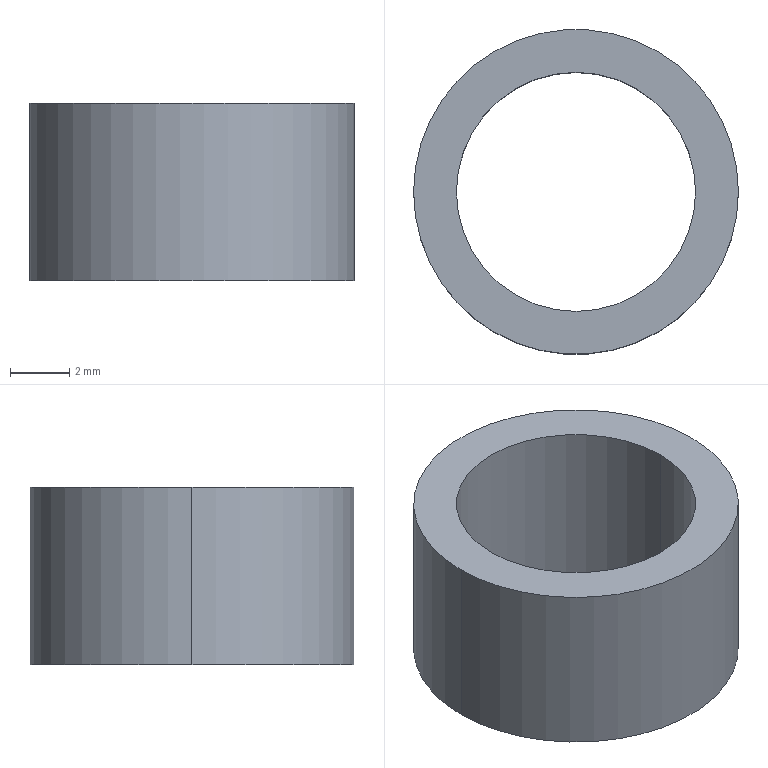Part | NX | features BREP 1 | 1 solid | 6 faces | box 11 x 11 x 6 mm | volume 261.019 mm3 | cylinder 4 | plane 2 | commonest cylinder face diameters 8.1 x2 11 x2
STEP:
#1=CARTESIAN_POINT('',(4.05,0.,6.));
#2=VERTEX_POINT('',#1);
#3=CARTESIAN_POINT('',(4.05,0.,0.));
#4=VERTEX_POINT('',#3);
#5=CARTESIAN_POINT('',(4.05,0.,6.));
#6=DIRECTION('',(0.,0.,-1.));
#7=VECTOR('',#6,1000.);
#8=LINE('',#5,#7);
#9=EDGE_CURVE('',#2,#4,#8,.T.);
#10=ORIENTED_EDGE('',*,*,#9,.F.);
#11=CARTESIAN_POINT('',(-4.05,0.,6.));
#12=VERTEX_POINT('',#11);
#13=CARTESIAN_POINT('',(0.,0.,6.));
#14=DIRECTION('',(0.,0.,1.));
#15=DIRECTION('',(1.,0.,0.));
#16=AXIS2_PLACEMENT_3D('',#13,#14,#15);
#17=CIRCLE('',#16,4.05);
#18=EDGE_CURVE('',#2,#12,#17,.T.);
#19=ORIENTED_EDGE('',*,*,#18,.T.);
#20=CARTESIAN_POINT('',(-4.05,0.,0.));
#21=VERTEX_POINT('',#20);
#22=CARTESIAN_POINT('',(-4.05,0.,6.));
#23=DIRECTION('',(0.,0.,-1.));
#24=VECTOR('',#23,1000.);
#25=LINE('',#22,#24);
#26=EDGE_CURVE('',#12,#21,#25,.T.);
#27=ORIENTED_EDGE('',*,*,#26,.T.);
#28=CARTESIAN_POINT('',(0.,0.,0.));
#29=DIRECTION('',(0.,0.,1.));
#30=DIRECTION('',(1.,0.,0.));
#31=AXIS2_PLACEMENT_3D('',#28,#29,#30);
#32=CIRCLE('',#31,4.05);
#33=EDGE_CURVE('',#4,#21,#32,.T.);
#34=ORIENTED_EDGE('',*,*,#33,.F.);
#35=EDGE_LOOP('',(#10,#19,#27,#34));
#36=FACE_BOUND('',#35,.T.);
#37=CARTESIAN_POINT('',(0.,0.,6.));
#38=DIRECTION('',(0.,0.,-1.));
#39=DIRECTION('',(-1.,0.,0.));
#40=AXIS2_PLACEMENT_3D('',#37,#38,#39);
#41=CYLINDRICAL_SURFACE('',#40,4.05);
#42=ADVANCED_FACE('',(#36),#41,.F.);
#43=CARTESIAN_POINT('',(5.5,0.,6.));
#44=VERTEX_POINT('',#43);
#45=CARTESIAN_POINT('',(5.5,0.,0.));
#46=VERTEX_POINT('',#45);
#47=CARTESIAN_POINT('',(5.5,0.,6.));
#48=DIRECTION('',(0.,0.,-1.));
#49=VECTOR('',#48,1000.);
#50=LINE('',#47,#49);
#51=EDGE_CURVE('',#44,#46,#50,.T.);
#52=ORIENTED_EDGE('',*,*,#51,.F.);
#53=CARTESIAN_POINT('',(-5.5,0.,6.));
#54=VERTEX_POINT('',#53);
#55=CARTESIAN_POINT('',(0.,0.,6.));
#56=DIRECTION('',(0.,0.,1.));
#57=DIRECTION('',(1.,0.,0.));
#58=AXIS2_PLACEMENT_3D('',#55,#56,#57);
#59=CIRCLE('',#58,5.5);
#60=EDGE_CURVE('',#54,#44,#59,.T.);
#61=ORIENTED_EDGE('',*,*,#60,.F.);
#62=CARTESIAN_POINT('',(-5.5,0.,0.));
#63=VERTEX_POINT('',#62);
#64=CARTESIAN_POINT('',(-5.5,0.,6.));
#65=DIRECTION('',(0.,0.,-1.));
#66=VECTOR('',#65,1000.);
#67=LINE('',#64,#66);
#68=EDGE_CURVE('',#54,#63,#67,.T.);
#69=ORIENTED_EDGE('',*,*,#68,.T.);
#70=CARTESIAN_POINT('',(0.,0.,0.));
#71=DIRECTION('',(0.,0.,1.));
#72=DIRECTION('',(1.,0.,0.));
#73=AXIS2_PLACEMENT_3D('',#70,#71,#72);
#74=CIRCLE('',#73,5.5);
#75=EDGE_CURVE('',#63,#46,#74,.T.);
#76=ORIENTED_EDGE('',*,*,#75,.T.);
#77=EDGE_LOOP('',(#52,#61,#69,#76));
#78=FACE_BOUND('',#77,.T.);
#79=CARTESIAN_POINT('',(0.,0.,6.));
#80=DIRECTION('',(0.,0.,-1.));
#81=DIRECTION('',(-1.,0.,0.));
#82=AXIS2_PLACEMENT_3D('',#79,#80,#81);
#83=CYLINDRICAL_SURFACE('',#82,5.5);
#84=ADVANCED_FACE('',(#78),#83,.T.);
#85=CARTESIAN_POINT('',(0.,0.,0.));
#86=DIRECTION('',(0.,0.,1.));
#87=DIRECTION('',(1.,0.,0.));
#88=AXIS2_PLACEMENT_3D('',#85,#86,#87);
#89=CIRCLE('',#88,4.05);
#90=EDGE_CURVE('',#21,#4,#89,.T.);
#91=ORIENTED_EDGE('',*,*,#90,.T.);
#92=ORIENTED_EDGE('',*,*,#33,.T.);
#93=EDGE_LOOP('',(#91,#92));
#94=FACE_BOUND('',#93,.T.);
#95=ORIENTED_EDGE('',*,*,#75,.F.);
#96=CARTESIAN_POINT('',(0.,0.,0.));
#97=DIRECTION('',(0.,0.,1.));
#98=DIRECTION('',(1.,0.,0.));
#99=AXIS2_PLACEMENT_3D('',#96,#97,#98);
#100=CIRCLE('',#99,5.5);
#101=EDGE_CURVE('',#46,#63,#100,.T.);
#102=ORIENTED_EDGE('',*,*,#101,.F.);
#103=EDGE_LOOP('',(#95,#102));
#104=FACE_BOUND('',#103,.T.);
#105=CARTESIAN_POINT('',(0.,0.,0.));
#106=DIRECTION('',(0.,0.,1.));
#107=DIRECTION('',(1.,0.,0.));
#108=AXIS2_PLACEMENT_3D('',#105,#106,#107);
#109=PLANE('',#108);
#110=ADVANCED_FACE('',(#94,#104),#109,.F.);
#111=CARTESIAN_POINT('',(0.,0.,6.));
#112=DIRECTION('',(0.,0.,1.));
#113=DIRECTION('',(1.,0.,0.));
#114=AXIS2_PLACEMENT_3D('',#111,#112,#113);
#115=CIRCLE('',#114,4.05);
#116=EDGE_CURVE('',#12,#2,#115,.T.);
#117=ORIENTED_EDGE('',*,*,#116,.F.);
#118=ORIENTED_EDGE('',*,*,#18,.F.);
#119=EDGE_LOOP('',(#117,#118));
#120=FACE_BOUND('',#119,.T.);
#121=ORIENTED_EDGE('',*,*,#60,.T.);
#122=CARTESIAN_POINT('',(0.,0.,6.));
#123=DIRECTION('',(0.,0.,1.));
#124=DIRECTION('',(1.,0.,0.));
#125=AXIS2_PLACEMENT_3D('',#122,#123,#124);
#126=CIRCLE('',#125,5.5);
#127=EDGE_CURVE('',#44,#54,#126,.T.);
#128=ORIENTED_EDGE('',*,*,#127,.T.);
#129=EDGE_LOOP('',(#121,#128));
#130=FACE_BOUND('',#129,.T.);
#131=CARTESIAN_POINT('',(0.,0.,6.));
#132=DIRECTION('',(0.,0.,1.));
#133=DIRECTION('',(1.,0.,0.));
#134=AXIS2_PLACEMENT_3D('',#131,#132,#133);
#135=PLANE('',#134);
#136=ADVANCED_FACE('',(#120,#130),#135,.T.);
#137=ORIENTED_EDGE('',*,*,#127,.F.);
#138=ORIENTED_EDGE('',*,*,#51,.T.);
#139=ORIENTED_EDGE('',*,*,#101,.T.);
#140=ORIENTED_EDGE('',*,*,#68,.F.);
#141=EDGE_LOOP('',(#137,#138,#139,#140));
#142=FACE_BOUND('',#141,.T.);
#143=CARTESIAN_POINT('',(0.,0.,6.));
#144=DIRECTION('',(0.,0.,-1.));
#145=DIRECTION('',(-1.,0.,0.));
#146=AXIS2_PLACEMENT_3D('',#143,#144,#145);
#147=CYLINDRICAL_SURFACE('',#146,5.5);
#148=ADVANCED_FACE('',(#142),#147,.T.);
#149=ORIENTED_EDGE('',*,*,#116,.T.);
#150=ORIENTED_EDGE('',*,*,#9,.T.);
#151=ORIENTED_EDGE('',*,*,#90,.F.);
#152=ORIENTED_EDGE('',*,*,#26,.F.);
#153=EDGE_LOOP('',(#149,#150,#151,#152));
#154=FACE_BOUND('',#153,.T.);
#155=CARTESIAN_POINT('',(0.,0.,6.));
#156=DIRECTION('',(0.,0.,-1.));
#157=DIRECTION('',(-1.,0.,0.));
#158=AXIS2_PLACEMENT_3D('',#155,#156,#157);
#159=CYLINDRICAL_SURFACE('',#158,4.05);
#160=ADVANCED_FACE('',(#154),#159,.F.);
#161=CLOSED_SHELL('',(#42,#84,#110,#136,#148,#160));
#162=MANIFOLD_SOLID_BREP('',#161);
#163=(LENGTH_UNIT()NAMED_UNIT(*)SI_UNIT(.MILLI.,.METRE.));
#164=UNCERTAINTY_MEASURE_WITH_UNIT(LENGTH_MEASURE(0.00001),#163,'','');
#165=(NAMED_UNIT(*)PLANE_ANGLE_UNIT()SI_UNIT($,.RADIAN.));
#166=(NAMED_UNIT(*)SI_UNIT($,.STERADIAN.)SOLID_ANGLE_UNIT());
#167=(GEOMETRIC_REPRESENTATION_CONTEXT(3)GLOBAL_UNCERTAINTY_ASSIGNED_CONTEXT((#164))GLOBAL_UNIT_ASSIGNED_CONTEXT((#163,#165,#166))REPRESENTATION_CONTEXT('',''));
#168=ADVANCED_BREP_SHAPE_REPRESENTATION('',(#162),#167);